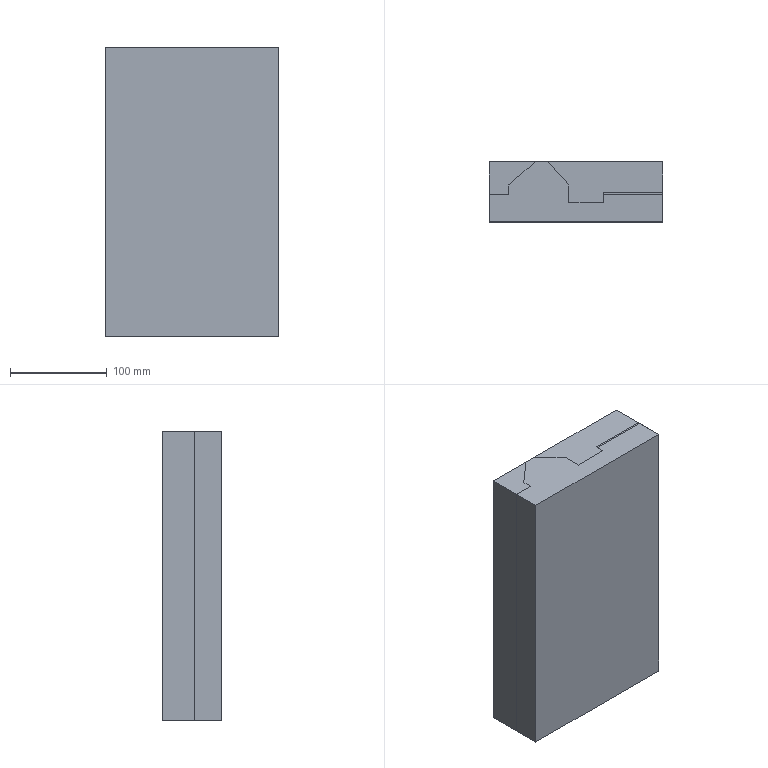NC program | NX | posted with a generic post | part box 180 x 62 x 300 mm
Lines 24929 to 25703 of 29776:
(定轴曲面加工 , TOOL : D17R0.8圆鼻飞刀)
N49850 T15 M6
N49852 /M1
N49854 G54
N49856 G17 G0 G90 X158.47 Y-77.7 S2000 M3
N49858 G43 Z20. H15
N49860 Z-15.674
N49862 G94 G1 X158.397 Z-16.784 F1400.
N49864 X158.18 Z-17.874
N49866 X157.823 Z-18.927
N49868 X157.331 Z-19.924
N49870 X156.713 Z-20.849
N49872 X155.98 Z-21.685
N49874 X155.144 Z-22.418
N49876 X154.22 Z-23.035
N49878 X153.223 Z-23.527
N49880 X152.17 Z-23.885
N49882 X151.079 Z-24.101
N49884 X149.97 Z-24.174
N49886 X-149.87 F2000.
N49888 X-149.915 Y-77.692 Z-24.167
N49890 X-149.95 Y-77.67 Z-24.148
N49892 X-149.97 Y-77.65 Z-24.13
N49894 Y-77.645 Z-24.126
N49896 X-149.943 Y-77.618 Z-24.101
N49898 X-149.922 Y-77.605 Z-24.09
N49900 X-149.895 Y-77.6 Z-24.086
N49902 X149.879
N49904 X149.916 Y-77.594 Z-24.08
N49906 X149.944 Y-77.576 Z-24.064
N49908 X149.968 Y-77.552 Z-24.043
N49910 X149.97 Y-77.548 Z-24.039
N49912 X149.968 Y-77.543 Z-24.035
N49914 X149.955 Y-77.53 Z-24.024
N49916 X149.92 Y-77.508 Z-24.004
N49918 X149.875 Y-77.5 Z-23.997
N49920 X-149.87
N49922 X-149.915 Y-77.492 Z-23.99
N49924 X-149.95 Y-77.47 Z-23.971
N49926 X-149.97 Y-77.45 Z-23.953
N49928 Y-77.445 Z-23.949
N49930 X-149.955 Y-77.43 Z-23.936
N49932 X-149.92 Y-77.408 Z-23.916
N49934 X-149.875 Y-77.4 Z-23.909
N49936 X149.879
N49938 X149.916 Y-77.394 Z-23.903
N49940 X149.944 Y-77.376 Z-23.888
N49942 X149.968 Y-77.352 Z-23.867
N49944 X149.97 Y-77.348 Z-23.863
N49946 X149.968 Y-77.343 Z-23.859
N49948 X149.955 Y-77.33 Z-23.847
N49950 X149.92 Y-77.308 Z-23.828
N49952 X149.875 Y-77.3 Z-23.821
N49954 X-149.87
N49956 X-149.915 Y-77.293 Z-23.814
N49958 X-149.95 Y-77.27 Z-23.794
N49960 X-149.97 Y-77.25 Z-23.777
N49962 Y-77.245 Z-23.772
N49964 X-149.943 Y-77.218 Z-23.748
N49966 X-149.922 Y-77.205 Z-23.736
N49968 X-149.895 Y-77.201 Z-23.732
N49970 X149.879
N49972 X149.916 Y-77.194 Z-23.727
N49974 X149.944 Y-77.176 Z-23.711
N49976 X149.968 Y-77.153 Z-23.69
N49978 X149.97 Y-77.148 Z-23.686
N49980 X149.968 Y-77.144 Z-23.682
N49982 X149.955 Y-77.131 Z-23.671
N49984 X149.92 Y-77.109 Z-23.651
N49986 X149.875 Y-77.101 Z-23.644
N49988 X-149.87
N49990 X-149.915 Y-77.093 Z-23.637
N49992 X-149.95 Y-77.071 Z-23.617
N49994 X-149.97 Y-77.051 Z-23.6
N49996 Y-77.046 Z-23.595
N49998 X-149.955 Y-77.031 Z-23.582
N50000 X-149.92 Y-77.009 Z-23.563
N50002 X-149.875 Y-77.001 Z-23.556
N50004 X149.879
N50006 X149.916 Y-76.994 Z-23.55
N50008 X149.944 Y-76.976 Z-23.534
N50010 X149.968 Y-76.953 Z-23.513
N50012 X149.97 Y-76.948 Z-23.509
N50014 X149.968 Y-76.944 Z-23.505
N50016 X149.955 Y-76.931 Z-23.494
N50018 X149.92 Y-76.909 Z-23.474
N50020 X149.875 Y-76.901 Z-23.467
N50022 X-149.87
N50024 X-149.915 Y-76.893 Z-23.46
N50026 X-149.95 Y-76.871 Z-23.441
N50028 X-149.97 Y-76.851 Z-23.423
N50030 Y-76.846 Z-23.419
N50032 X-149.943 Y-76.819 Z-23.395
N50034 X-149.922 Y-76.806 Z-23.383
N50036 X-149.895 Y-76.801 Z-23.379
N50038 X149.879
N50040 X149.916 Y-76.795 Z-23.373
N50042 X149.944 Y-76.777 Z-23.357
N50044 X149.968 Y-76.753 Z-23.336
N50046 X149.97 Y-76.749 Z-23.333
N50048 X149.968 Y-76.744 Z-23.329
N50050 X149.955 Y-76.731 Z-23.317
N50052 X149.92 Y-76.709 Z-23.298
N50054 X149.875 Y-76.701 Z-23.291
N50056 X-149.87
N50058 X-149.915 Y-76.693 Z-23.284
N50060 X-149.95 Y-76.671 Z-23.264
N50062 X-149.97 Y-76.651 Z-23.246
N50064 Y-76.646 Z-23.242
N50066 X-149.955 Y-76.631 Z-23.229
N50068 X-149.92 Y-76.609 Z-23.209
N50070 X-149.875 Y-76.601 Z-23.202
N50072 X149.879
N50074 X149.916 Y-76.595 Z-23.196
N50076 X149.944 Y-76.577 Z-23.181
N50078 X149.968 Y-76.553 Z-23.16
N50080 X149.97 Y-76.549 Z-23.156
N50082 X149.968 Y-76.544 Z-23.152
N50084 X149.955 Y-76.531 Z-23.14
N50086 X149.92 Y-76.509 Z-23.121
N50088 X149.875 Y-76.501 Z-23.114
N50090 X-149.87
N50092 X-149.915 Y-76.493 Z-23.107
N50094 X-149.95 Y-76.471 Z-23.087
N50096 X-149.97 Y-76.451 Z-23.07
N50098 Y-76.446 Z-23.065
N50100 X-149.955 Y-76.431 Z-23.052
N50102 X-149.92 Y-76.409 Z-23.032
N50104 X-149.875 Y-76.401 Z-23.025
N50106 X149.879
N50108 X149.916 Y-76.395 Z-23.02
N50110 X149.944 Y-76.377 Z-23.004
N50112 X149.968 Y-76.354 Z-22.983
N50114 X149.97 Y-76.349 Z-22.979
N50116 X149.968 Y-76.345 Z-22.975
N50118 X149.955 Y-76.332 Z-22.964
N50120 X149.92 Y-76.31 Z-22.944
N50122 X149.875 Y-76.302 Z-22.937
N50124 X-149.87
N50126 X-149.915 Y-76.294 Z-22.93
N50128 X-149.95 Y-76.272 Z-22.911
N50130 X-149.97 Y-76.252 Z-22.893
N50132 Y-76.247 Z-22.888
N50134 X-149.943 Y-76.219 Z-22.864
N50136 X-149.922 Y-76.206 Z-22.853
N50138 X-149.895 Y-76.202 Z-22.849
N50140 X149.879
N50142 X149.916 Y-76.195 Z-22.843
N50144 X149.944 Y-76.177 Z-22.827
N50146 X149.968 Y-76.154 Z-22.806
N50148 X149.97 Y-76.149 Z-22.802
N50150 X149.968 Y-76.145 Z-22.798
N50152 X149.955 Y-76.132 Z-22.787
N50154 X149.92 Y-76.11 Z-22.767
N50156 X149.875 Y-76.102 Z-22.76
N50158 X-149.87
N50160 X-149.915 Y-76.094 Z-22.753
N50162 X-149.95 Y-76.072 Z-22.734
N50164 X-149.97 Y-76.052 Z-22.716
N50166 Y-76.047 Z-22.712
N50168 X-149.955 Y-76.032 Z-22.698
N50170 X-149.92 Y-76.01 Z-22.679
N50172 X-149.875 Y-76.002 Z-22.672
N50174 X149.879
N50176 X149.916 Y-75.996 Z-22.666
N50178 X149.944 Y-75.978 Z-22.65
N50180 X149.968 Y-75.954 Z-22.63
N50182 X149.97 Y-75.95 Z-22.626
N50184 X149.968 Y-75.945 Z-22.622
N50186 X149.955 Y-75.932 Z-22.61
N50188 X149.92 Y-75.91 Z-22.591
N50190 X149.875 Y-75.902 Z-22.584
N50192 X-149.87
N50194 X-149.915 Y-75.894 Z-22.577
N50196 X-149.95 Y-75.872 Z-22.557
N50198 X-149.97 Y-75.852 Z-22.539
N50200 Y-75.847 Z-22.535
N50202 X-149.955 Y-75.832 Z-22.522
N50204 X-149.92 Y-75.81 Z-22.502
N50206 X-149.875 Y-75.802 Z-22.495
N50208 X149.879
N50210 X149.916 Y-75.796 Z-22.49
N50212 X149.944 Y-75.778 Z-22.474
N50214 X149.968 Y-75.754 Z-22.453
N50216 X149.97 Y-75.75 Z-22.449
N50218 X149.968 Y-75.745 Z-22.445
N50220 X149.955 Y-75.732 Z-22.433
N50222 X149.92 Y-75.71 Z-22.414
N50224 X149.875 Y-75.702 Z-22.407
N50226 X-149.87
N50228 X-149.915 Y-75.694 Z-22.4
N50230 X-149.95 Y-75.672 Z-22.38
N50232 X-149.97 Y-75.652 Z-22.363
N50234 Y-75.647 Z-22.358
N50236 X-149.955 Y-75.632 Z-22.345
N50238 X-149.92 Y-75.61 Z-22.325
N50240 X-149.875 Y-75.602 Z-22.318
N50242 X149.879
N50244 X149.916 Y-75.596 Z-22.313
N50246 X149.944 Y-75.578 Z-22.297
N50248 X149.968 Y-75.554 Z-22.276
N50250 X149.97 Y-75.55 Z-22.272
N50252 X149.968 Y-75.546 Z-22.268
N50254 X149.955 Y-75.533 Z-22.257
N50256 X149.92 Y-75.51 Z-22.237
N50258 X149.875 Y-75.503 Z-22.23
N50260 X-149.87
N50262 X-149.915 Y-75.495 Z-22.223
N50264 X-149.95 Y-75.473 Z-22.204
N50266 X-149.97 Y-75.453 Z-22.186
N50268 Y-75.448 Z-22.182
N50270 X-149.955 Y-75.433 Z-22.168
N50272 X-149.92 Y-75.411 Z-22.149
N50274 X-149.875 Y-75.403 Z-22.142
N50276 X149.879
N50278 X149.916 Y-75.396 Z-22.136
N50280 X149.944 Y-75.378 Z-22.12
N50282 X149.968 Y-75.355 Z-22.099
N50284 X149.97 Y-75.35 Z-22.095
N50286 X149.968 Y-75.346 Z-22.091
N50288 X149.955 Y-75.333 Z-22.08
N50290 X149.92 Y-75.311 Z-22.06
N50292 X149.875 Y-75.303 Z-22.053
N50294 X-149.87
N50296 X-149.915 Y-75.295 Z-22.046
N50298 X-149.95 Y-75.273 Z-22.027
N50300 X-149.97 Y-75.253 Z-22.009
N50302 Y-75.248 Z-22.005
N50304 X-149.955 Y-75.233 Z-21.992
N50306 X-149.92 Y-75.211 Z-21.972
N50308 X-149.875 Y-75.203 Z-21.965
N50310 X149.879
N50312 X149.916 Y-75.196 Z-21.959
N50314 X149.944 Y-75.179 Z-21.944
N50316 X149.968 Y-75.155 Z-21.923
N50318 X149.97 Y-75.151 Z-21.919
N50320 X149.968 Y-75.146 Z-21.915
N50322 X149.955 Y-75.133 Z-21.903
N50324 X149.92 Y-75.111 Z-21.884
N50326 X149.875 Y-75.103 Z-21.877
N50328 X-149.87
N50330 X-149.915 Y-75.095 Z-21.87
N50332 X-149.95 Y-75.073 Z-21.85
N50334 X-149.97 Y-75.053 Z-21.832
N50336 Y-75.048 Z-21.828
N50338 X-149.943 Y-75.021 Z-21.804
N50340 X-149.922 Y-75.008 Z-21.792
N50342 X-149.895 Y-75.003 Z-21.788
N50344 X149.879
N50346 X149.916 Y-74.997 Z-21.783
N50348 X149.944 Y-74.979 Z-21.767
N50350 X149.968 Y-74.955 Z-21.746
N50352 X149.97 Y-74.951 Z-21.742
N50354 X149.968 Y-74.946 Z-21.738
N50356 X149.955 Y-74.933 Z-21.726
N50358 X149.92 Y-74.911 Z-21.707
N50360 X149.875 Y-74.903 Z-21.7
N50362 X-149.87
N50364 X-149.915 Y-74.895 Z-21.693
N50366 X-149.95 Y-74.873 Z-21.673
N50368 X-149.97 Y-74.853 Z-21.656
N50370 Y-74.848 Z-21.651
N50372 X-149.943 Y-74.821 Z-21.627
N50374 X-149.922 Y-74.808 Z-21.616
N50376 X-149.895 Y-74.803 Z-21.612
N50378 X149.879
N50380 X149.916 Y-74.797 Z-21.606
N50382 X149.944 Y-74.779 Z-21.59
N50384 X149.968 Y-74.755 Z-21.569
N50386 X149.97 Y-74.751 Z-21.565
N50388 X149.968 Y-74.746 Z-21.561
N50390 X149.955 Y-74.733 Z-21.55
N50392 X149.92 Y-74.711 Z-21.53
N50394 X149.875 Y-74.703 Z-21.523
N50396 X-149.87
N50398 X-149.915 Y-74.696 Z-21.516
N50400 X-149.95 Y-74.673 Z-21.497
N50402 X-149.97 Y-74.654 Z-21.479
N50404 Y-74.649 Z-21.475
N50406 X-149.943 Y-74.621 Z-21.451
N50408 X-149.922 Y-74.608 Z-21.439
N50410 X-149.895 Y-74.604 Z-21.435
N50412 X149.879
N50414 X149.916 Y-74.597 Z-21.429
N50416 X149.944 Y-74.579 Z-21.413
N50418 X149.968 Y-74.556 Z-21.392
N50420 X149.97 Y-74.551 Z-21.388
N50422 X149.968 Y-74.547 Z-21.385
N50424 X149.955 Y-74.534 Z-21.373
N50426 X149.92 Y-74.512 Z-21.353
N50428 X149.875 Y-74.504 Z-21.346
N50430 X-149.87
N50432 X-149.915 Y-74.496 Z-21.339
N50434 X-149.95 Y-74.474 Z-21.32
N50436 X-149.97 Y-74.454 Z-21.302
N50438 Y-74.449 Z-21.298
N50440 X-149.943 Y-74.422 Z-21.274
N50442 X-149.922 Y-74.409 Z-21.262
N50444 X-149.895 Y-74.404 Z-21.258
N50446 X149.879
N50448 X149.916 Y-74.397 Z-21.252
N50450 X149.944 Y-74.38 Z-21.237
N50452 X149.968 Y-74.356 Z-21.216
N50454 X149.97 Y-74.351 Z-21.212
N50456 X149.968 Y-74.347 Z-21.208
N50458 X149.955 Y-74.334 Z-21.196
N50460 X149.92 Y-74.312 Z-21.177
N50462 X149.875 Y-74.304 Z-21.17
N50464 X-149.87
N50466 X-149.915 Y-74.296 Z-21.163
N50468 X-149.95 Y-74.274 Z-21.143
N50470 X-149.97 Y-74.254 Z-21.126
N50472 Y-74.249 Z-21.121
N50474 X-149.943 Y-74.222 Z-21.097
N50476 X-149.922 Y-74.209 Z-21.086
N50478 X-149.895 Y-74.204 Z-21.081
N50480 X149.879
N50482 X149.916 Y-74.198 Z-21.076
N50484 X149.944 Y-74.18 Z-21.06
N50486 X149.968 Y-74.156 Z-21.039
N50488 X149.97 Y-74.152 Z-21.035
N50490 X149.968 Y-74.147 Z-21.031
N50492 X149.955 Y-74.134 Z-21.02
N50494 X149.92 Y-74.112 Z-21.
N50496 X149.875 Y-74.104 Z-20.993
N50498 X-149.87
N50500 X-149.915 Y-74.096 Z-20.986
N50502 X-149.95 Y-74.074 Z-20.966
N50504 X-149.97 Y-74.054 Z-20.949
N50506 Y-74.049 Z-20.944
N50508 X-149.943 Y-74.022 Z-20.92
N50510 X-149.922 Y-74.009 Z-20.909
N50512 X-149.895 Y-74.004 Z-20.905
N50514 X149.879
N50516 X149.916 Y-73.998 Z-20.899
N50518 X149.944 Y-73.98 Z-20.883
N50520 X149.968 Y-73.956 Z-20.862
N50522 X149.97 Y-73.952 Z-20.858
N50524 X149.968 Y-73.947 Z-20.854
N50526 X149.955 Y-73.934 Z-20.843
N50528 X149.92 Y-73.912 Z-20.823
N50530 X149.875 Y-73.904 Z-20.816
N50532 X-149.87
N50534 X-149.915 Y-73.897 Z-20.809
N50536 X-149.95 Y-73.874 Z-20.79
N50538 X-149.97 Y-73.855 Z-20.772
N50540 Y-73.85 Z-20.768
N50542 X-149.955 Y-73.835 Z-20.754
N50544 X-149.92 Y-73.812 Z-20.735
N50546 X-149.875 Y-73.805 Z-20.728
N50548 X149.879
N50550 X149.916 Y-73.798 Z-20.722
N50552 X149.944 Y-73.78 Z-20.706
N50554 X149.968 Y-73.757 Z-20.685
N50556 X149.97 Y-73.752 Z-20.682
N50558 X149.968 Y-73.748 Z-20.678
N50560 X149.955 Y-73.735 Z-20.666
N50562 X149.92 Y-73.713 Z-20.647
N50564 X149.875 Y-73.705 Z-20.64
N50566 X-149.87
N50568 X-149.915 Y-73.697 Z-20.633
N50570 X-149.95 Y-73.675 Z-20.613
N50572 X-149.97 Y-73.655 Z-20.595
N50574 Y-73.65 Z-20.591
N50576 X-149.955 Y-73.635 Z-20.578
N50578 X-149.92 Y-73.613 Z-20.558
N50580 X-149.875 Y-73.605 Z-20.551
N50582 X149.879
N50584 X149.916 Y-73.598 Z-20.546
N50586 X149.944 Y-73.581 Z-20.53
N50588 X149.968 Y-73.557 Z-20.509
N50590 X149.97 Y-73.552 Z-20.505
N50592 X149.968 Y-73.548 Z-20.501
N50594 X149.955 Y-73.535 Z-20.489
N50596 X149.92 Y-73.513 Z-20.47
N50598 X149.875 Y-73.505 Z-20.463
N50600 X-149.87
N50602 X-149.915 Y-73.497 Z-20.456
N50604 X-149.95 Y-73.475 Z-20.436
N50606 X-149.97 Y-73.455 Z-20.419
N50608 Y-73.45 Z-20.414
N50610 X-149.955 Y-73.435 Z-20.401
N50612 X-149.92 Y-73.413 Z-20.381
N50614 X-149.875 Y-73.405 Z-20.374
N50616 X149.879
N50618 X149.916 Y-73.399 Z-20.369
N50620 X149.944 Y-73.381 Z-20.353
N50622 X149.968 Y-73.357 Z-20.332
N50624 X149.97 Y-73.353 Z-20.328
N50626 X149.968 Y-73.348 Z-20.324
N50628 X149.955 Y-73.335 Z-20.313
N50630 X149.92 Y-73.313 Z-20.293
N50632 X149.875 Y-73.305 Z-20.286
N50634 X-149.87
N50636 X-149.915 Y-73.297 Z-20.279
N50638 X-149.95 Y-73.275 Z-20.26
N50640 X-149.97 Y-73.255 Z-20.242
N50642 Y-73.25 Z-20.237
N50644 X-149.955 Y-73.235 Z-20.224
N50646 X-149.92 Y-73.213 Z-20.205
N50648 X-149.875 Y-73.205 Z-20.198
N50650 X149.879
N50652 X149.916 Y-73.199 Z-20.192
N50654 X149.944 Y-73.181 Z-20.176
N50656 X149.968 Y-73.157 Z-20.155
N50658 X149.97 Y-73.153 Z-20.151
N50660 X149.968 Y-73.148 Z-20.147
N50662 X149.955 Y-73.135 Z-20.136
N50664 X149.92 Y-73.113 Z-20.116
N50666 X149.875 Y-73.105 Z-20.109
N50668 X-149.87
N50670 X-149.915 Y-73.097 Z-20.102
N50672 X-149.95 Y-73.075 Z-20.083
N50674 X-149.97 Y-73.055 Z-20.065
N50676 Y-73.05 Z-20.061
N50678 X-149.955 Y-73.036 Z-20.048
N50680 X-149.92 Y-73.013 Z-20.028
N50682 X-149.875 Y-73.006 Z-20.021
N50684 X149.879
N50686 X149.916 Y-72.999 Z-20.015
N50688 X149.944 Y-72.981 Z-20.
N50690 X149.968 Y-72.958 Z-19.979
N50692 X149.97 Y-72.953 Z-19.975
N50694 X149.968 Y-72.949 Z-19.971
N50696 X149.955 Y-72.936 Z-19.959
N50698 X149.92 Y-72.914 Z-19.94
N50700 X149.875 Y-72.906 Z-19.933
N50702 X-149.87
N50704 X-149.915 Y-72.898 Z-19.926
N50706 X-149.95 Y-72.876 Z-19.906
N50708 X-149.97 Y-72.856 Z-19.888
N50710 Y-72.851 Z-19.884
N50712 X-149.955 Y-72.836 Z-19.871
N50714 X-149.92 Y-72.814 Z-19.851
N50716 X-149.875 Y-72.806 Z-19.844
N50718 X149.879
N50720 X149.916 Y-72.799 Z-19.839
N50722 X149.944 Y-72.781 Z-19.823
N50724 X149.968 Y-72.758 Z-19.802
N50726 X149.97 Y-72.753 Z-19.798
N50728 X149.968 Y-72.749 Z-19.794
N50730 X149.955 Y-72.736 Z-19.782
N50732 X149.92 Y-72.714 Z-19.763
N50734 X149.875 Y-72.706 Z-19.756
N50736 X-149.87
N50738 X-149.915 Y-72.698 Z-19.749
N50740 X-149.95 Y-72.676 Z-19.729
N50742 X-149.97 Y-72.656 Z-19.712
N50744 Y-72.651 Z-19.707
N50746 X-149.955 Y-72.636 Z-19.694
N50748 X-149.92 Y-72.614 Z-19.675
N50750 X-149.875 Y-72.606 Z-19.668
N50752 X149.879
N50754 X149.916 Y-72.6 Z-19.662
N50756 X149.944 Y-72.582 Z-19.646
N50758 X149.968 Y-72.558 Z-19.625
N50760 X149.97 Y-72.554 Z-19.621
N50762 X149.968 Y-72.549 Z-19.617
N50764 X149.955 Y-72.536 Z-19.606
N50766 X149.92 Y-72.514 Z-19.586
N50768 X149.875 Y-72.506 Z-19.579
N50770 X-149.87
N50772 X-149.915 Y-72.498 Z-19.572
N50774 X-149.95 Y-72.476 Z-19.553
N50776 X-149.97 Y-72.456 Z-19.535
N50778 Y-72.451 Z-19.531
N50780 X-149.955 Y-72.436 Z-19.517
N50782 X-149.92 Y-72.414 Z-19.498
N50784 X-149.875 Y-72.406 Z-19.491
N50786 X149.879
N50788 X149.916 Y-72.4 Z-19.485
N50790 X149.944 Y-72.382 Z-19.469
N50792 X149.968 Y-72.358 Z-19.448
N50794 X149.97 Y-72.354 Z-19.444
N50796 X149.968 Y-72.349 Z-19.44
N50798 X149.955 Y-72.336 Z-19.429
N50800 X149.92 Y-72.314 Z-19.409
N50802 X149.875 Y-72.306 Z-19.402
N50804 X-149.87
N50806 X-149.915 Y-72.298 Z-19.395
N50808 X-149.95 Y-72.276 Z-19.376
N50810 X-149.97 Y-72.256 Z-19.358
N50812 Y-72.251 Z-19.354
N50814 X-149.943 Y-72.224 Z-19.33
N50816 X-149.922 Y-72.211 Z-19.318
N50818 X-149.895 Y-72.206 Z-19.314
N50820 X149.879
N50822 X149.916 Y-72.2 Z-19.308
N50824 X149.944 Y-72.182 Z-19.293
N50826 X149.968 Y-72.158 Z-19.272
N50828 X149.97 Y-72.154 Z-19.268
N50830 X149.968 Y-72.15 Z-19.264
N50832 X149.955 Y-72.137 Z-19.252
N50834 X149.92 Y-72.114 Z-19.233
N50836 X149.875 Y-72.107 Z-19.226
N50838 X-149.87
N50840 X-149.915 Y-72.099 Z-19.219
N50842 X-149.95 Y-72.077 Z-19.199
N50844 X-149.97 Y-72.057 Z-19.182
N50846 Y-72.052 Z-19.177
N50848 X-149.955 Y-72.037 Z-19.164
N50850 X-149.92 Y-72.015 Z-19.144
N50852 X-149.875 Y-72.007 Z-19.137
N50854 X149.879
N50856 X149.916 Y-72. Z-19.132
N50858 X149.944 Y-71.982 Z-19.116
N50860 X149.968 Y-71.959 Z-19.095
N50862 X149.97 Y-71.954 Z-19.091
N50864 X149.968 Y-71.95 Z-19.087
N50866 X149.955 Y-71.937 Z-19.076
N50868 X149.92 Y-71.915 Z-19.056
N50870 X149.875 Y-71.907 Z-19.049
N50872 X-149.87
N50874 X-149.915 Y-71.899 Z-19.042
N50876 X-149.95 Y-71.877 Z-19.022
N50878 X-149.97 Y-71.857 Z-19.005
N50880 Y-71.852 Z-19.
N50882 X-149.943 Y-71.825 Z-18.976
N50884 X-149.922 Y-71.812 Z-18.965
N50886 X-149.895 Y-71.807 Z-18.961
N50888 X149.879
N50890 X149.916 Y-71.801 Z-18.955
N50892 X149.944 Y-71.783 Z-18.939
N50894 X149.968 Y-71.759 Z-18.918
N50896 X149.97 Y-71.755 Z-18.914
N50898 X149.968 Y-71.75 Z-18.91
N50900 X149.955 Y-71.737 Z-18.899
N50902 X149.92 Y-71.715 Z-18.879
N50904 X149.875 Y-71.707 Z-18.872
N50906 X-149.87
N50908 X-149.915 Y-71.699 Z-18.865
N50910 X-149.95 Y-71.677 Z-18.846
N50912 X-149.97 Y-71.657 Z-18.828
N50914 Y-71.652 Z-18.824
N50916 X-149.955 Y-71.637 Z-18.81
N50918 X-149.92 Y-71.615 Z-18.791
N50920 X-149.875 Y-71.607 Z-18.784
N50922 X149.879
N50924 X149.916 Y-71.601 Z-18.778
N50926 X149.944 Y-71.583 Z-18.762
N50928 X149.968 Y-71.559 Z-18.741
N50930 X149.97 Y-71.555 Z-18.738
N50932 X149.968 Y-71.55 Z-18.734
N50934 X149.955 Y-71.537 Z-18.722
N50936 X149.92 Y-71.515 Z-18.703
N50938 X149.875 Y-71.507 Z-18.696
N50940 X-149.87
N50942 X-149.915 Y-71.499 Z-18.689
N50944 X-149.95 Y-71.477 Z-18.669
N50946 X-149.97 Y-71.457 Z-18.651
N50948 Y-71.452 Z-18.647
N50950 X-149.955 Y-71.437 Z-18.634
N50952 X-149.92 Y-71.415 Z-18.614
N50954 X-149.875 Y-71.407 Z-18.607
N50956 X149.879
N50958 X149.916 Y-71.401 Z-18.601
N50960 X149.944 Y-71.383 Z-18.586
N50962 X149.968 Y-71.359 Z-18.565
N50964 X149.97 Y-71.355 Z-18.561
N50966 X149.968 Y-71.351 Z-18.557
N50968 X149.955 Y-71.338 Z-18.545
N50970 X149.92 Y-71.315 Z-18.526
N50972 X149.875 Y-71.308 Z-18.519
N50974 X-149.87
N50976 X-149.915 Y-71.3 Z-18.512
N50978 X-149.95 Y-71.278 Z-18.492
N50980 X-149.97 Y-71.258 Z-18.475
N50982 Y-71.253 Z-18.47
N50984 X-149.955 Y-71.238 Z-18.457
N50986 X-149.92 Y-71.216 Z-18.437
N50988 X-149.875 Y-71.208 Z-18.43
N50990 X149.879
N50992 X149.916 Y-71.201 Z-18.425
N50994 X149.944 Y-71.183 Z-18.409
N50996 X149.968 Y-71.16 Z-18.388
N50998 X149.97 Y-71.155 Z-18.384
N51000 X149.968 Y-71.151 Z-18.38
N51002 X149.955 Y-71.138 Z-18.369
N51004 X149.92 Y-71.116 Z-18.349
N51006 X149.875 Y-71.108 Z-18.342
N51008 X-149.87
N51010 X-149.915 Y-71.1 Z-18.335
N51012 X-149.95 Y-71.078 Z-18.316
N51014 X-149.97 Y-71.058 Z-18.298
N51016 Y-71.053 Z-18.293
N51018 X-149.955 Y-71.038 Z-18.28
N51020 X-149.92 Y-71.016 Z-18.261
N51022 X-149.875 Y-71.008 Z-18.254
N51024 X149.879
N51026 X149.916 Y-71.001 Z-18.248
N51028 X149.944 Y-70.984 Z-18.232
N51030 X149.968 Y-70.96 Z-18.211
N51032 X149.97 Y-70.955 Z-18.207
N51034 X149.968 Y-70.951 Z-18.203
N51036 X149.955 Y-70.938 Z-18.192
N51038 X149.92 Y-70.916 Z-18.172
N51040 X149.875 Y-70.908 Z-18.165
N51042 X-149.87
N51044 X-149.915 Y-70.9 Z-18.158
N51046 X-149.95 Y-70.878 Z-18.139
N51048 X-149.97 Y-70.858 Z-18.121
N51050 Y-70.853 Z-18.117
N51052 X-149.943 Y-70.826 Z-18.093
N51054 X-149.922 Y-70.813 Z-18.081
N51056 X-149.895 Y-70.808 Z-18.077
N51058 X149.879
N51060 X149.916 Y-70.802 Z-18.071
N51062 X149.944 Y-70.784 Z-18.055
N51064 X149.968 Y-70.76 Z-18.035
N51066 X149.97 Y-70.756 Z-18.031
N51068 X149.968 Y-70.751 Z-18.027
N51070 X149.955 Y-70.738 Z-18.015
N51072 X149.92 Y-70.716 Z-17.996
N51074 X149.875 Y-70.708 Z-17.989
N51076 X-149.87
N51078 X-149.915 Y-70.7 Z-17.982
N51080 X-149.95 Y-70.678 Z-17.962
N51082 X-149.97 Y-70.658 Z-17.944
N51084 Y-70.653 Z-17.94
N51086 X-149.955 Y-70.638 Z-17.927
N51088 X-149.92 Y-70.616 Z-17.907
N51090 X-149.875 Y-70.608 Z-17.9
N51092 X149.879
N51094 X149.916 Y-70.602 Z-17.895
N51096 X149.944 Y-70.584 Z-17.879
N51098 X149.968 Y-70.56 Z-17.858
N51100 X149.97 Y-70.556 Z-17.854
N51102 X149.968 Y-70.551 Z-17.85
N51104 X149.955 Y-70.538 Z-17.838
N51106 X149.92 Y-70.516 Z-17.819
N51108 X149.875 Y-70.508 Z-17.812
N51110 X-149.87
N51112 X-149.915 Y-70.501 Z-17.805
N51114 X-149.95 Y-70.478 Z-17.785
N51116 X-149.97 Y-70.459 Z-17.768
N51118 Y-70.454 Z-17.763
N51120 X-149.955 Y-70.439 Z-17.75
N51122 X-149.92 Y-70.417 Z-17.731
N51124 X-149.875 Y-70.409 Z-17.724
N51126 X149.879
N51128 X149.916 Y-70.402 Z-17.718
N51130 X149.944 Y-70.384 Z-17.702
N51132 X149.968 Y-70.361 Z-17.681
N51134 X149.97 Y-70.356 Z-17.677
N51136 X149.968 Y-70.352 Z-17.673
N51138 X149.955 Y-70.339 Z-17.662
N51140 X149.92 Y-70.317 Z-17.642
N51142 X149.875 Y-70.309 Z-17.635
N51144 X-149.87
N51146 X-149.915 Y-70.301 Z-17.628
N51148 X-149.95 Y-70.279 Z-17.609
N51150 X-149.97 Y-70.259 Z-17.591
N51152 Y-70.254 Z-17.587
N51154 X-149.955 Y-70.239 Z-17.573
N51156 X-149.92 Y-70.217 Z-17.554
N51158 X-149.875 Y-70.209 Z-17.547
N51160 X149.879
N51162 X149.916 Y-70.202 Z-17.541
N51164 X149.944 Y-70.185 Z-17.525
N51166 X149.968 Y-70.161 Z-17.504
N51168 X149.97 Y-70.156 Z-17.5
N51170 X149.968 Y-70.152 Z-17.496
N51172 X149.955 Y-70.139 Z-17.485
N51174 X149.92 Y-70.117 Z-17.465
N51176 X149.875 Y-70.109 Z-17.458
N51178 X-149.87
N51180 X-149.915 Y-70.101 Z-17.451
N51182 X-149.95 Y-70.079 Z-17.432
N51184 X-149.97 Y-70.059 Z-17.414
N51186 Y-70.054 Z-17.41
N51188 X-149.943 Y-70.027 Z-17.386
N51190 X-149.922 Y-70.014 Z-17.374
N51192 X-149.895 Y-70.009 Z-17.37
N51194 X149.879
N51196 X149.916 Y-70.003 Z-17.364
N51198 X149.944 Y-69.985 Z-17.349
N51200 X149.968 Y-69.961 Z-17.328
N51202 X149.97 Y-69.957 Z-17.324
N51204 X149.968 Y-69.952 Z-17.32
N51206 X149.955 Y-69.939 Z-17.308
N51208 X149.92 Y-69.917 Z-17.289
N51210 X149.875 Y-69.909 Z-17.282
N51212 X-149.87
N51214 X-149.915 Y-69.901 Z-17.275
N51216 X-149.95 Y-69.879 Z-17.255
N51218 X-149.97 Y-69.859 Z-17.237
N51220 Y-69.854 Z-17.233
N51222 X-149.943 Y-69.827 Z-17.209
N51224 X-149.922 Y-69.814 Z-17.197
N51226 X-149.895 Y-69.809 Z-17.193
N51228 X149.879
N51230 X149.916 Y-69.803 Z-17.188
N51232 X149.944 Y-69.785 Z-17.172
N51234 X149.968 Y-69.761 Z-17.151
N51236 X149.97 Y-69.757 Z-17.147
N51238 X149.968 Y-69.752 Z-17.143
N51240 X149.955 Y-69.739 Z-17.131
N51242 X149.92 Y-69.717 Z-17.112
N51244 X149.875 Y-69.709 Z-17.105
N51246 X-149.87
N51248 X-149.915 Y-69.701 Z-17.098
N51250 X-149.95 Y-69.679 Z-17.078
N51252 X-149.97 Y-69.659 Z-17.061
N51254 Y-69.654 Z-17.056
N51256 X-149.955 Y-69.64 Z-17.043
N51258 X-149.92 Y-69.617 Z-17.024
N51260 X-149.875 Y-69.61 Z-17.017
N51262 X149.879
N51264 X149.916 Y-69.603 Z-17.011
N51266 X149.944 Y-69.585 Z-16.995
N51268 X149.968 Y-69.562 Z-16.974
N51270 X149.97 Y-69.557 Z-16.97
N51272 X149.968 Y-69.553 Z-16.966
N51274 X149.955 Y-69.54 Z-16.955
N51276 X149.92 Y-69.518 Z-16.935
N51278 X149.875 Y-69.51 Z-16.928
N51280 X-149.87
N51282 X-149.915 Y-69.502 Z-16.921
N51284 X-149.95 Y-69.48 Z-16.902
N51286 X-149.97 Y-69.46 Z-16.884
N51288 Y-69.455 Z-16.88
N51290 X-149.955 Y-69.44 Z-16.866
N51292 X-149.92 Y-69.418 Z-16.847
N51294 X-149.875 Y-69.41 Z-16.84
N51296 X149.879
N51298 X149.916 Y-69.403 Z-16.834
N51300 X149.944 Y-69.385 Z-16.818
N51302 X149.968 Y-69.362 Z-16.797
N51304 X149.97 Y-69.357 Z-16.793
N51306 X149.968 Y-69.353 Z-16.79
N51308 X149.955 Y-69.34 Z-16.778
N51310 X149.92 Y-69.318 Z-16.758
N51312 X149.875 Y-69.31 Z-16.751
N51314 X-149.87
N51316 X-149.915 Y-69.302 Z-16.744
N51318 X-149.95 Y-69.28 Z-16.725
N51320 X-149.97 Y-69.26 Z-16.707
N51322 Y-69.255 Z-16.703
N51324 X-149.955 Y-69.24 Z-16.69
N51326 X-149.92 Y-69.218 Z-16.67
N51328 X-149.875 Y-69.21 Z-16.663
N51330 X149.879
N51332 X149.916 Y-69.204 Z-16.657
N51334 X149.944 Y-69.186 Z-16.642
N51336 X149.968 Y-69.162 Z-16.621
N51338 X149.97 Y-69.158 Z-16.617
N51340 X149.968 Y-69.153 Z-16.613
N51342 X149.955 Y-69.14 Z-16.601
N51344 X149.92 Y-69.118 Z-16.582
N51346 X149.875 Y-69.11 Z-16.575
N51348 X-149.87
N51350 X-149.915 Y-69.102 Z-16.568
N51352 X-149.95 Y-69.08 Z-16.548
N51354 X-149.97 Y-69.06 Z-16.531
N51356 Y-69.055 Z-16.526
N51358 X-149.955 Y-69.04 Z-16.513
N51360 X-149.92 Y-69.018 Z-16.493
N51362 X-149.875 Y-69.01 Z-16.486
N51364 X149.879
N51366 X149.916 Y-69.004 Z-16.481
N51368 X149.944 Y-68.986 Z-16.465
N51370 X149.968 Y-68.962 Z-16.444
N51372 X149.97 Y-68.958 Z-16.44
N51374 X149.968 Y-68.953 Z-16.436
N51376 X149.955 Y-68.94 Z-16.425
N51378 X149.92 Y-68.918 Z-16.405
N51380 X149.875 Y-68.91 Z-16.398
N51382 X-149.87
N51384 X-149.915 Y-68.902 Z-16.391
N51386 X-149.95 Y-68.88 Z-16.371
N51388 X-149.97 Y-68.86 Z-16.354
N51390 Y-68.855 Z-16.349
N51392 X-149.943 Y-68.828 Z-16.325